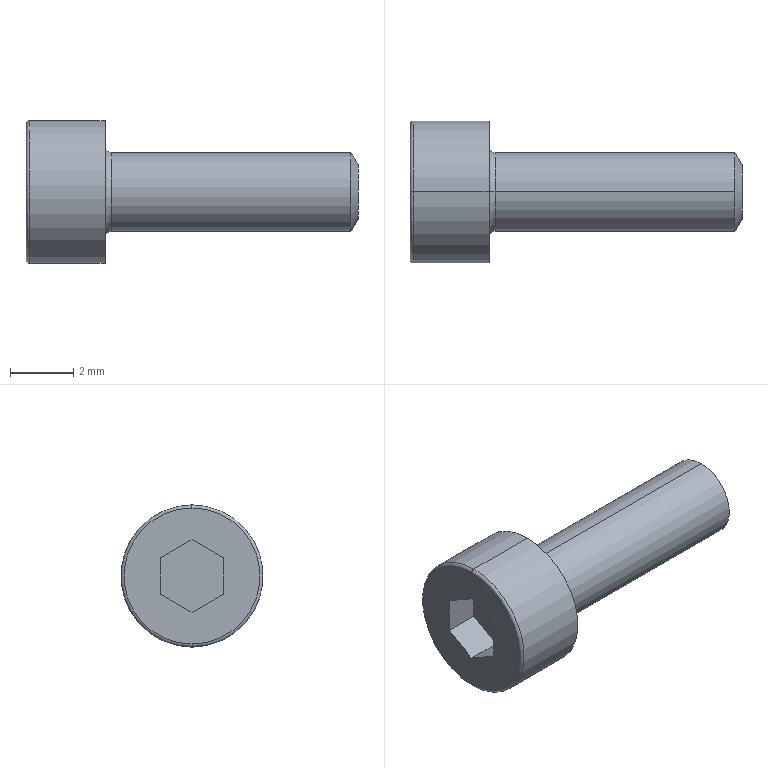Part | SolidWorks | features BlendCut 1, Cut 1, Fillet 1, LPattern 1, RevCut 1, Revolution 1 | 1 solid | 20 faces | box 10.5 x 4.5 x 4.5 mm | volume 74.982 mm3 | plane 10 | torus 4 | cylinder 4 | cone 2 | commonest cylinder face diameters 2.5 x2 4.5 x2
STEP:
#1=CARTESIAN_POINT('',(0.,0.,2.15));
#2=VERTEX_POINT('',#1);
#3=CARTESIAN_POINT('',(0.,0.,-2.15));
#4=VERTEX_POINT('',#3);
#5=CARTESIAN_POINT('',(0.,0.,0.));
#6=DIRECTION('',(-1.,0.,0.));
#7=DIRECTION('',(0.,0.,-1.));
#8=AXIS2_PLACEMENT_3D('',#5,#6,#7);
#9=CIRCLE('',#8,2.15);
#10=EDGE_CURVE('',#2,#4,#9,.T.);
#11=ORIENTED_EDGE('',*,*,#10,.F.);
#12=CARTESIAN_POINT('',(0.1,0.,2.25));
#13=VERTEX_POINT('',#12);
#14=CARTESIAN_POINT('',(0.1,0.,2.15));
#15=DIRECTION('',(0.,1.,0.));
#16=DIRECTION('',(0.,0.,1.));
#17=AXIS2_PLACEMENT_3D('',#14,#15,#16);
#18=CIRCLE('',#17,0.1);
#19=EDGE_CURVE('',#2,#13,#18,.T.);
#20=ORIENTED_EDGE('',*,*,#19,.T.);
#21=CARTESIAN_POINT('',(0.1,0.,-2.25));
#22=VERTEX_POINT('',#21);
#23=CARTESIAN_POINT('',(0.1,0.,0.));
#24=DIRECTION('',(1.,0.,0.));
#25=DIRECTION('',(0.,0.,-1.));
#26=AXIS2_PLACEMENT_3D('',#23,#24,#25);
#27=CIRCLE('',#26,2.25);
#28=EDGE_CURVE('',#22,#13,#27,.T.);
#29=ORIENTED_EDGE('',*,*,#28,.F.);
#30=CARTESIAN_POINT('',(0.1,0.,-2.15));
#31=DIRECTION('',(0.,-1.,0.));
#32=DIRECTION('',(0.,0.,-1.));
#33=AXIS2_PLACEMENT_3D('',#30,#31,#32);
#34=CIRCLE('',#33,0.1);
#35=EDGE_CURVE('',#4,#22,#34,.T.);
#36=ORIENTED_EDGE('',*,*,#35,.F.);
#37=EDGE_LOOP('',(#11,#20,#29,#36));
#38=FACE_OUTER_BOUND('',#37,.T.);
#39=CARTESIAN_POINT('',(0.1,0.,0.));
#40=DIRECTION('',(1.,0.,0.));
#41=DIRECTION('',(0.,0.,-1.));
#42=AXIS2_PLACEMENT_3D('',#39,#40,#41);
#43=TOROIDAL_SURFACE('',#42,2.15,0.1);
#44=ADVANCED_FACE('',(#38),#43,.T.);
#45=CARTESIAN_POINT('',(10.5,0.,0.8603));
#46=VERTEX_POINT('',#45);
#47=CARTESIAN_POINT('',(10.5,0.,-0.8603));
#48=VERTEX_POINT('',#47);
#49=CARTESIAN_POINT('',(10.5,0.,0.));
#50=DIRECTION('',(-1.,0.,0.));
#51=DIRECTION('',(0.,0.,1.));
#52=AXIS2_PLACEMENT_3D('',#49,#50,#51);
#53=CIRCLE('',#52,0.8603);
#54=EDGE_CURVE('',#46,#48,#53,.T.);
#55=ORIENTED_EDGE('',*,*,#54,.T.);
#56=CARTESIAN_POINT('',(10.275,0.,-1.25));
#57=VERTEX_POINT('',#56);
#58=CARTESIAN_POINT('',(10.275,0.,-1.25));
#59=DIRECTION('',(-0.5,0.,-0.866));
#60=VECTOR('',#59,1000.);
#61=LINE('',#58,#60);
#62=EDGE_CURVE('',#48,#57,#61,.T.);
#63=ORIENTED_EDGE('',*,*,#62,.T.);
#64=CARTESIAN_POINT('',(10.275,0.,1.25));
#65=VERTEX_POINT('',#64);
#66=CARTESIAN_POINT('',(10.275,0.,0.));
#67=DIRECTION('',(-1.,0.,0.));
#68=DIRECTION('',(0.,0.,1.));
#69=AXIS2_PLACEMENT_3D('',#66,#67,#68);
#70=CIRCLE('',#69,1.25);
#71=EDGE_CURVE('',#65,#57,#70,.T.);
#72=ORIENTED_EDGE('',*,*,#71,.F.);
#73=CARTESIAN_POINT('',(10.275,0.,1.25));
#74=DIRECTION('',(-0.5,0.,0.866));
#75=VECTOR('',#74,1000.);
#76=LINE('',#73,#75);
#77=EDGE_CURVE('',#46,#65,#76,.T.);
#78=ORIENTED_EDGE('',*,*,#77,.F.);
#79=EDGE_LOOP('',(#55,#63,#72,#78));
#80=FACE_OUTER_BOUND('',#79,.T.);
#81=CARTESIAN_POINT('',(10.275,0.,0.));
#82=DIRECTION('',(-1.,0.,0.));
#83=DIRECTION('',(0.,0.,1.));
#84=AXIS2_PLACEMENT_3D('',#81,#82,#83);
#85=CONICAL_SURFACE('',#84,1.25,1.047);
#86=ADVANCED_FACE('',(#80),#85,.T.);
#87=CARTESIAN_POINT('',(2.5,0.,-1.45));
#88=VERTEX_POINT('',#87);
#89=CARTESIAN_POINT('',(2.5,0.,1.45));
#90=VERTEX_POINT('',#89);
#91=CARTESIAN_POINT('',(2.5,0.,0.));
#92=DIRECTION('',(-1.,0.,0.));
#93=DIRECTION('',(0.,0.,1.));
#94=AXIS2_PLACEMENT_3D('',#91,#92,#93);
#95=CIRCLE('',#94,1.45);
#96=EDGE_CURVE('',#88,#90,#95,.T.);
#97=ORIENTED_EDGE('',*,*,#96,.F.);
#98=CARTESIAN_POINT('',(2.7,0.,-1.25));
#99=VERTEX_POINT('',#98);
#100=CARTESIAN_POINT('',(2.7,0.,-1.45));
#101=DIRECTION('',(0.,1.,0.));
#102=DIRECTION('',(0.,0.,1.));
#103=AXIS2_PLACEMENT_3D('',#100,#101,#102);
#104=CIRCLE('',#103,0.2);
#105=EDGE_CURVE('',#88,#99,#104,.T.);
#106=ORIENTED_EDGE('',*,*,#105,.T.);
#107=CARTESIAN_POINT('',(2.7,0.,1.25));
#108=VERTEX_POINT('',#107);
#109=CARTESIAN_POINT('',(2.7,0.,0.));
#110=DIRECTION('',(-1.,0.,0.));
#111=DIRECTION('',(0.,0.,1.));
#112=AXIS2_PLACEMENT_3D('',#109,#110,#111);
#113=CIRCLE('',#112,1.25);
#114=EDGE_CURVE('',#99,#108,#113,.T.);
#115=ORIENTED_EDGE('',*,*,#114,.T.);
#116=CARTESIAN_POINT('',(2.7,0.,1.45));
#117=DIRECTION('',(0.,-1.,0.));
#118=DIRECTION('',(0.,0.,-1.));
#119=AXIS2_PLACEMENT_3D('',#116,#117,#118);
#120=CIRCLE('',#119,0.2);
#121=EDGE_CURVE('',#90,#108,#120,.T.);
#122=ORIENTED_EDGE('',*,*,#121,.F.);
#123=EDGE_LOOP('',(#97,#106,#115,#122));
#124=FACE_OUTER_BOUND('',#123,.T.);
#125=CARTESIAN_POINT('',(2.7,0.,0.));
#126=DIRECTION('',(-1.,0.,0.));
#127=DIRECTION('',(0.,0.,1.));
#128=AXIS2_PLACEMENT_3D('',#125,#126,#127);
#129=TOROIDAL_SURFACE('',#128,1.45,0.2);
#130=ADVANCED_FACE('',(#124),#129,.F.);
#131=CARTESIAN_POINT('',(2.5,0.,2.25));
#132=VERTEX_POINT('',#131);
#133=CARTESIAN_POINT('',(2.5,0.,-2.25));
#134=VERTEX_POINT('',#133);
#135=CARTESIAN_POINT('',(2.5,0.,0.));
#136=DIRECTION('',(-1.,0.,0.));
#137=DIRECTION('',(0.,0.,1.));
#138=AXIS2_PLACEMENT_3D('',#135,#136,#137);
#139=CIRCLE('',#138,2.25);
#140=EDGE_CURVE('',#132,#134,#139,.T.);
#141=ORIENTED_EDGE('',*,*,#140,.T.);
#142=CARTESIAN_POINT('',(0.,0.,-2.25));
#143=DIRECTION('',(-1.,0.,0.));
#144=VECTOR('',#143,1000.);
#145=LINE('',#142,#144);
#146=EDGE_CURVE('',#134,#22,#145,.T.);
#147=ORIENTED_EDGE('',*,*,#146,.T.);
#148=ORIENTED_EDGE('',*,*,#28,.T.);
#149=CARTESIAN_POINT('',(0.,0.,2.25));
#150=DIRECTION('',(-1.,0.,0.));
#151=VECTOR('',#150,1000.);
#152=LINE('',#149,#151);
#153=EDGE_CURVE('',#132,#13,#152,.T.);
#154=ORIENTED_EDGE('',*,*,#153,.F.);
#155=EDGE_LOOP('',(#141,#147,#148,#154));
#156=FACE_OUTER_BOUND('',#155,.T.);
#157=CARTESIAN_POINT('',(0.,0.,0.));
#158=DIRECTION('',(-1.,0.,0.));
#159=DIRECTION('',(0.,0.,1.));
#160=AXIS2_PLACEMENT_3D('',#157,#158,#159);
#161=CYLINDRICAL_SURFACE('',#160,2.25);
#162=ADVANCED_FACE('',(#156),#161,.T.);
#163=ORIENTED_EDGE('',*,*,#71,.T.);
#164=CARTESIAN_POINT('',(0.,0.,-1.25));
#165=DIRECTION('',(-1.,0.,0.));
#166=VECTOR('',#165,1000.);
#167=LINE('',#164,#166);
#168=EDGE_CURVE('',#57,#99,#167,.T.);
#169=ORIENTED_EDGE('',*,*,#168,.T.);
#170=CARTESIAN_POINT('',(2.7,0.,0.));
#171=DIRECTION('',(-1.,0.,0.));
#172=DIRECTION('',(0.,0.,1.));
#173=AXIS2_PLACEMENT_3D('',#170,#171,#172);
#174=CIRCLE('',#173,1.25);
#175=EDGE_CURVE('',#108,#99,#174,.T.);
#176=ORIENTED_EDGE('',*,*,#175,.F.);
#177=CARTESIAN_POINT('',(0.,0.,1.25));
#178=DIRECTION('',(-1.,0.,0.));
#179=VECTOR('',#178,1000.);
#180=LINE('',#177,#179);
#181=EDGE_CURVE('',#65,#108,#180,.T.);
#182=ORIENTED_EDGE('',*,*,#181,.F.);
#183=EDGE_LOOP('',(#163,#169,#176,#182));
#184=FACE_OUTER_BOUND('',#183,.T.);
#185=CARTESIAN_POINT('',(0.,0.,0.));
#186=DIRECTION('',(-1.,0.,0.));
#187=DIRECTION('',(0.,0.,1.));
#188=AXIS2_PLACEMENT_3D('',#185,#186,#187);
#189=CYLINDRICAL_SURFACE('',#188,1.25);
#190=ADVANCED_FACE('',(#184),#189,.T.);
#191=ORIENTED_EDGE('',*,*,#168,.F.);
#192=CARTESIAN_POINT('',(10.275,0.,0.));
#193=DIRECTION('',(-1.,0.,0.));
#194=DIRECTION('',(0.,0.,1.));
#195=AXIS2_PLACEMENT_3D('',#192,#193,#194);
#196=CIRCLE('',#195,1.25);
#197=EDGE_CURVE('',#57,#65,#196,.T.);
#198=ORIENTED_EDGE('',*,*,#197,.T.);
#199=ORIENTED_EDGE('',*,*,#181,.T.);
#200=ORIENTED_EDGE('',*,*,#114,.F.);
#201=EDGE_LOOP('',(#191,#198,#199,#200));
#202=FACE_OUTER_BOUND('',#201,.T.);
#203=CARTESIAN_POINT('',(0.,0.,0.));
#204=DIRECTION('',(-1.,0.,0.));
#205=DIRECTION('',(0.,0.,1.));
#206=AXIS2_PLACEMENT_3D('',#203,#204,#205);
#207=CYLINDRICAL_SURFACE('',#206,1.25);
#208=ADVANCED_FACE('',(#202),#207,.T.);
#209=CARTESIAN_POINT('',(0.,0.,0.));
#210=DIRECTION('',(-1.,0.,0.));
#211=DIRECTION('',(0.,0.,-1.));
#212=AXIS2_PLACEMENT_3D('',#209,#210,#211);
#213=CIRCLE('',#212,2.15);
#214=EDGE_CURVE('',#4,#2,#213,.T.);
#215=ORIENTED_EDGE('',*,*,#214,.T.);
#216=ORIENTED_EDGE('',*,*,#10,.T.);
#217=EDGE_LOOP('',(#215,#216));
#218=FACE_OUTER_BOUND('',#217,.T.);
#219=CARTESIAN_POINT('',(0.,0.,1.15));
#220=VERTEX_POINT('',#219);
#221=CARTESIAN_POINT('',(0.,0.9959,0.575));
#222=VERTEX_POINT('',#221);
#223=CARTESIAN_POINT('',(0.,0.,1.15));
#224=DIRECTION('',(0.,0.866,-0.5));
#225=VECTOR('',#224,1000.);
#226=LINE('',#223,#225);
#227=EDGE_CURVE('',#220,#222,#226,.T.);
#228=ORIENTED_EDGE('',*,*,#227,.F.);
#229=CARTESIAN_POINT('',(0.,-0.9959,0.575));
#230=VERTEX_POINT('',#229);
#231=CARTESIAN_POINT('',(0.,-0.9959,0.575));
#232=DIRECTION('',(0.,0.866,0.5));
#233=VECTOR('',#232,1000.);
#234=LINE('',#231,#233);
#235=EDGE_CURVE('',#230,#220,#234,.T.);
#236=ORIENTED_EDGE('',*,*,#235,.F.);
#237=CARTESIAN_POINT('',(0.,-0.9959,-0.575));
#238=VERTEX_POINT('',#237);
#239=CARTESIAN_POINT('',(0.,-0.9959,-0.575));
#240=DIRECTION('',(0.,0.,1.));
#241=VECTOR('',#240,1000.);
#242=LINE('',#239,#241);
#243=EDGE_CURVE('',#238,#230,#242,.T.);
#244=ORIENTED_EDGE('',*,*,#243,.F.);
#245=CARTESIAN_POINT('',(0.,0.,-1.15));
#246=VERTEX_POINT('',#245);
#247=CARTESIAN_POINT('',(0.,0.,-1.15));
#248=DIRECTION('',(0.,-0.866,0.5));
#249=VECTOR('',#248,1000.);
#250=LINE('',#247,#249);
#251=EDGE_CURVE('',#246,#238,#250,.T.);
#252=ORIENTED_EDGE('',*,*,#251,.F.);
#253=CARTESIAN_POINT('',(0.,0.9959,-0.575));
#254=VERTEX_POINT('',#253);
#255=CARTESIAN_POINT('',(0.,0.9959,-0.575));
#256=DIRECTION('',(0.,-0.866,-0.5));
#257=VECTOR('',#256,1000.);
#258=LINE('',#255,#257);
#259=EDGE_CURVE('',#254,#246,#258,.T.);
#260=ORIENTED_EDGE('',*,*,#259,.F.);
#261=CARTESIAN_POINT('',(0.,0.9959,0.575));
#262=DIRECTION('',(0.,0.,-1.));
#263=VECTOR('',#262,1000.);
#264=LINE('',#261,#263);
#265=EDGE_CURVE('',#222,#254,#264,.T.);
#266=ORIENTED_EDGE('',*,*,#265,.F.);
#267=EDGE_LOOP('',(#228,#236,#244,#252,#260,#266));
#268=FACE_BOUND('',#267,.T.);
#269=CARTESIAN_POINT('',(0.,0.,0.));
#270=DIRECTION('',(1.,0.,0.));
#271=DIRECTION('',(0.,0.,-1.));
#272=AXIS2_PLACEMENT_3D('',#269,#270,#271);
#273=PLANE('',#272);
#274=ADVANCED_FACE('',(#218,#268),#273,.F.);
#275=ORIENTED_EDGE('',*,*,#146,.F.);
#276=CARTESIAN_POINT('',(2.5,0.,0.));
#277=DIRECTION('',(-1.,0.,0.));
#278=DIRECTION('',(0.,0.,1.));
#279=AXIS2_PLACEMENT_3D('',#276,#277,#278);
#280=CIRCLE('',#279,2.25);
#281=EDGE_CURVE('',#134,#132,#280,.T.);
#282=ORIENTED_EDGE('',*,*,#281,.T.);
#283=ORIENTED_EDGE('',*,*,#153,.T.);
#284=CARTESIAN_POINT('',(0.1,0.,0.));
#285=DIRECTION('',(1.,0.,0.));
#286=DIRECTION('',(0.,0.,-1.));
#287=AXIS2_PLACEMENT_3D('',#284,#285,#286);
#288=CIRCLE('',#287,2.25);
#289=EDGE_CURVE('',#13,#22,#288,.T.);
#290=ORIENTED_EDGE('',*,*,#289,.T.);
#291=EDGE_LOOP('',(#275,#282,#283,#290));
#292=FACE_OUTER_BOUND('',#291,.T.);
#293=CARTESIAN_POINT('',(0.,0.,0.));
#294=DIRECTION('',(-1.,0.,0.));
#295=DIRECTION('',(0.,0.,1.));
#296=AXIS2_PLACEMENT_3D('',#293,#294,#295);
#297=CYLINDRICAL_SURFACE('',#296,2.25);
#298=ADVANCED_FACE('',(#292),#297,.T.);
#299=ORIENTED_EDGE('',*,*,#140,.F.);
#300=ORIENTED_EDGE('',*,*,#281,.F.);
#301=EDGE_LOOP('',(#299,#300));
#302=FACE_OUTER_BOUND('',#301,.T.);
#303=CARTESIAN_POINT('',(2.5,0.,0.));
#304=DIRECTION('',(-1.,0.,0.));
#305=DIRECTION('',(0.,0.,1.));
#306=AXIS2_PLACEMENT_3D('',#303,#304,#305);
#307=CIRCLE('',#306,1.45);
#308=EDGE_CURVE('',#90,#88,#307,.T.);
#309=ORIENTED_EDGE('',*,*,#308,.T.);
#310=ORIENTED_EDGE('',*,*,#96,.T.);
#311=EDGE_LOOP('',(#309,#310));
#312=FACE_BOUND('',#311,.T.);
#313=CARTESIAN_POINT('',(2.5,2.25,0.));
#314=DIRECTION('',(-1.,0.,0.));
#315=DIRECTION('',(0.,0.,1.));
#316=AXIS2_PLACEMENT_3D('',#313,#314,#315);
#317=PLANE('',#316);
#318=ADVANCED_FACE('',(#302,#312),#317,.F.);
#319=ORIENTED_EDGE('',*,*,#105,.F.);
#320=ORIENTED_EDGE('',*,*,#308,.F.);
#321=ORIENTED_EDGE('',*,*,#121,.T.);
#322=ORIENTED_EDGE('',*,*,#175,.T.);
#323=EDGE_LOOP('',(#319,#320,#321,#322));
#324=FACE_OUTER_BOUND('',#323,.T.);
#325=CARTESIAN_POINT('',(2.7,0.,0.));
#326=DIRECTION('',(-1.,0.,0.));
#327=DIRECTION('',(0.,0.,1.));
#328=AXIS2_PLACEMENT_3D('',#325,#326,#327);
#329=TOROIDAL_SURFACE('',#328,1.45,0.2);
#330=ADVANCED_FACE('',(#324),#329,.F.);
#331=ORIENTED_EDGE('',*,*,#235,.T.);
#332=CARTESIAN_POINT('',(1.1,0.,1.15));
#333=VERTEX_POINT('',#332);
#334=CARTESIAN_POINT('',(1.1,0.,1.15));
#335=DIRECTION('',(-1.,0.,0.));
#336=VECTOR('',#335,1000.);
#337=LINE('',#334,#336);
#338=EDGE_CURVE('',#333,#220,#337,.T.);
#339=ORIENTED_EDGE('',*,*,#338,.F.);
#340=CARTESIAN_POINT('',(1.1,-0.9959,0.575));
#341=VERTEX_POINT('',#340);
#342=CARTESIAN_POINT('',(1.1,-0.9959,0.575));
#343=DIRECTION('',(0.,0.866,0.5));
#344=VECTOR('',#343,1000.);
#345=LINE('',#342,#344);
#346=EDGE_CURVE('',#341,#333,#345,.T.);
#347=ORIENTED_EDGE('',*,*,#346,.F.);
#348=CARTESIAN_POINT('',(1.1,-0.9959,0.575));
#349=DIRECTION('',(-1.,0.,0.));
#350=VECTOR('',#349,1000.);
#351=LINE('',#348,#350);
#352=EDGE_CURVE('',#341,#230,#351,.T.);
#353=ORIENTED_EDGE('',*,*,#352,.T.);
#354=EDGE_LOOP('',(#331,#339,#347,#353));
#355=FACE_OUTER_BOUND('',#354,.T.);
#356=CARTESIAN_POINT('',(1.1,-0.9959,0.575));
#357=DIRECTION('',(0.,-0.5,0.866));
#358=DIRECTION('',(0.,-0.866,-0.5));
#359=AXIS2_PLACEMENT_3D('',#356,#357,#358);
#360=PLANE('',#359);
#361=ADVANCED_FACE('',(#355),#360,.F.);
#362=ORIENTED_EDGE('',*,*,#243,.T.);
#363=ORIENTED_EDGE('',*,*,#352,.F.);
#364=CARTESIAN_POINT('',(1.1,-0.9959,-0.575));
#365=VERTEX_POINT('',#364);
#366=CARTESIAN_POINT('',(1.1,-0.9959,-0.575));
#367=DIRECTION('',(0.,0.,1.));
#368=VECTOR('',#367,1000.);
#369=LINE('',#366,#368);
#370=EDGE_CURVE('',#365,#341,#369,.T.);
#371=ORIENTED_EDGE('',*,*,#370,.F.);
#372=CARTESIAN_POINT('',(1.1,-0.9959,-0.575));
#373=DIRECTION('',(-1.,0.,0.));
#374=VECTOR('',#373,1000.);
#375=LINE('',#372,#374);
#376=EDGE_CURVE('',#365,#238,#375,.T.);
#377=ORIENTED_EDGE('',*,*,#376,.T.);
#378=EDGE_LOOP('',(#362,#363,#371,#377));
#379=FACE_OUTER_BOUND('',#378,.T.);
#380=CARTESIAN_POINT('',(1.1,-0.9959,-0.575));
#381=DIRECTION('',(0.,-1.,0.));
#382=DIRECTION('',(0.,0.,-1.));
#383=AXIS2_PLACEMENT_3D('',#380,#381,#382);
#384=PLANE('',#383);
#385=ADVANCED_FACE('',(#379),#384,.F.);
#386=ORIENTED_EDGE('',*,*,#251,.T.);
#387=ORIENTED_EDGE('',*,*,#376,.F.);
#388=CARTESIAN_POINT('',(1.1,0.,-1.15));
#389=VERTEX_POINT('',#388);
#390=CARTESIAN_POINT('',(1.1,0.,-1.15));
#391=DIRECTION('',(0.,-0.866,0.5));
#392=VECTOR('',#391,1000.);
#393=LINE('',#390,#392);
#394=EDGE_CURVE('',#389,#365,#393,.T.);
#395=ORIENTED_EDGE('',*,*,#394,.F.);
#396=CARTESIAN_POINT('',(1.1,0.,-1.15));
#397=DIRECTION('',(-1.,0.,0.));
#398=VECTOR('',#397,1000.);
#399=LINE('',#396,#398);
#400=EDGE_CURVE('',#389,#246,#399,.T.);
#401=ORIENTED_EDGE('',*,*,#400,.T.);
#402=EDGE_LOOP('',(#386,#387,#395,#401));
#403=FACE_OUTER_BOUND('',#402,.T.);
#404=CARTESIAN_POINT('',(1.1,0.,-1.15));
#405=DIRECTION('',(0.,-0.5,-0.866));
#406=DIRECTION('',(0.,0.866,-0.5));
#407=AXIS2_PLACEMENT_3D('',#404,#405,#406);
#408=PLANE('',#407);
#409=ADVANCED_FACE('',(#403),#408,.F.);
#410=ORIENTED_EDGE('',*,*,#259,.T.);
#411=ORIENTED_EDGE('',*,*,#400,.F.);
#412=CARTESIAN_POINT('',(1.1,0.9959,-0.575));
#413=VERTEX_POINT('',#412);
#414=CARTESIAN_POINT('',(1.1,0.9959,-0.575));
#415=DIRECTION('',(0.,-0.866,-0.5));
#416=VECTOR('',#415,1000.);
#417=LINE('',#414,#416);
#418=EDGE_CURVE('',#413,#389,#417,.T.);
#419=ORIENTED_EDGE('',*,*,#418,.F.);
#420=CARTESIAN_POINT('',(1.1,0.9959,-0.575));
#421=DIRECTION('',(-1.,0.,0.));
#422=VECTOR('',#421,1000.);
#423=LINE('',#420,#422);
#424=EDGE_CURVE('',#413,#254,#423,.T.);
#425=ORIENTED_EDGE('',*,*,#424,.T.);
#426=EDGE_LOOP('',(#410,#411,#419,#425));
#427=FACE_OUTER_BOUND('',#426,.T.);
#428=CARTESIAN_POINT('',(1.1,0.9959,-0.575));
#429=DIRECTION('',(0.,0.5,-0.866));
#430=DIRECTION('',(0.,0.866,0.5));
#431=AXIS2_PLACEMENT_3D('',#428,#429,#430);
#432=PLANE('',#431);
#433=ADVANCED_FACE('',(#427),#432,.F.);
#434=ORIENTED_EDGE('',*,*,#265,.T.);
#435=ORIENTED_EDGE('',*,*,#424,.F.);
#436=CARTESIAN_POINT('',(1.1,0.9959,0.575));
#437=VERTEX_POINT('',#436);
#438=CARTESIAN_POINT('',(1.1,0.9959,0.575));
#439=DIRECTION('',(0.,0.,-1.));
#440=VECTOR('',#439,1000.);
#441=LINE('',#438,#440);
#442=EDGE_CURVE('',#437,#413,#441,.T.);
#443=ORIENTED_EDGE('',*,*,#442,.F.);
#444=CARTESIAN_POINT('',(1.1,0.9959,0.575));
#445=DIRECTION('',(-1.,0.,0.));
#446=VECTOR('',#445,1000.);
#447=LINE('',#444,#446);
#448=EDGE_CURVE('',#437,#222,#447,.T.);
#449=ORIENTED_EDGE('',*,*,#448,.T.);
#450=EDGE_LOOP('',(#434,#435,#443,#449));
#451=FACE_OUTER_BOUND('',#450,.T.);
#452=CARTESIAN_POINT('',(1.1,0.9959,0.575));
#453=DIRECTION('',(0.,1.,0.));
#454=DIRECTION('',(0.,0.,1.));
#455=AXIS2_PLACEMENT_3D('',#452,#453,#454);
#456=PLANE('',#455);
#457=ADVANCED_FACE('',(#451),#456,.F.);
#458=ORIENTED_EDGE('',*,*,#227,.T.);
#459=ORIENTED_EDGE('',*,*,#448,.F.);
#460=CARTESIAN_POINT('',(1.1,0.,1.15));
#461=DIRECTION('',(0.,0.866,-0.5));
#462=VECTOR('',#461,1000.);
#463=LINE('',#460,#462);
#464=EDGE_CURVE('',#333,#437,#463,.T.);
#465=ORIENTED_EDGE('',*,*,#464,.F.);
#466=ORIENTED_EDGE('',*,*,#338,.T.);
#467=EDGE_LOOP('',(#458,#459,#465,#466));
#468=FACE_OUTER_BOUND('',#467,.T.);
#469=CARTESIAN_POINT('',(1.1,0.,1.15));
#470=DIRECTION('',(0.,0.5,0.866));
#471=DIRECTION('',(0.,-0.866,0.5));
#472=AXIS2_PLACEMENT_3D('',#469,#470,#471);
#473=PLANE('',#472);
#474=ADVANCED_FACE('',(#468),#473,.F.);
#475=ORIENTED_EDGE('',*,*,#346,.T.);
#476=ORIENTED_EDGE('',*,*,#464,.T.);
#477=ORIENTED_EDGE('',*,*,#442,.T.);
#478=ORIENTED_EDGE('',*,*,#418,.T.);
#479=ORIENTED_EDGE('',*,*,#394,.T.);
#480=ORIENTED_EDGE('',*,*,#370,.T.);
#481=EDGE_LOOP('',(#475,#476,#477,#478,#479,#480));
#482=FACE_OUTER_BOUND('',#481,.T.);
#483=CARTESIAN_POINT('',(1.1,-0.9959,0.575));
#484=DIRECTION('',(1.,0.,0.));
#485=DIRECTION('',(0.,0.,-1.));
#486=AXIS2_PLACEMENT_3D('',#483,#484,#485);
#487=PLANE('',#486);
#488=ADVANCED_FACE('',(#482),#487,.F.);
#489=ORIENTED_EDGE('',*,*,#62,.F.);
#490=CARTESIAN_POINT('',(10.5,0.,0.));
#491=DIRECTION('',(-1.,0.,0.));
#492=DIRECTION('',(0.,0.,1.));
#493=AXIS2_PLACEMENT_3D('',#490,#491,#492);
#494=CIRCLE('',#493,0.8603);
#495=EDGE_CURVE('',#48,#46,#494,.T.);
#496=ORIENTED_EDGE('',*,*,#495,.T.);
#497=ORIENTED_EDGE('',*,*,#77,.T.);
#498=ORIENTED_EDGE('',*,*,#197,.F.);
#499=EDGE_LOOP('',(#489,#496,#497,#498));
#500=FACE_OUTER_BOUND('',#499,.T.);
#501=CARTESIAN_POINT('',(10.275,0.,0.));
#502=DIRECTION('',(-1.,0.,0.));
#503=DIRECTION('',(0.,0.,1.));
#504=AXIS2_PLACEMENT_3D('',#501,#502,#503);
#505=CONICAL_SURFACE('',#504,1.25,1.047);
#506=ADVANCED_FACE('',(#500),#505,.T.);
#507=ORIENTED_EDGE('',*,*,#54,.F.);
#508=ORIENTED_EDGE('',*,*,#495,.F.);
#509=EDGE_LOOP('',(#507,#508));
#510=FACE_OUTER_BOUND('',#509,.T.);
#511=CARTESIAN_POINT('',(10.5,1.25,0.));
#512=DIRECTION('',(-1.,0.,0.));
#513=DIRECTION('',(0.,0.,1.));
#514=AXIS2_PLACEMENT_3D('',#511,#512,#513);
#515=PLANE('',#514);
#516=ADVANCED_FACE('',(#510),#515,.F.);
#517=ORIENTED_EDGE('',*,*,#19,.F.);
#518=ORIENTED_EDGE('',*,*,#214,.F.);
#519=ORIENTED_EDGE('',*,*,#35,.T.);
#520=ORIENTED_EDGE('',*,*,#289,.F.);
#521=EDGE_LOOP('',(#517,#518,#519,#520));
#522=FACE_OUTER_BOUND('',#521,.T.);
#523=CARTESIAN_POINT('',(0.1,0.,0.));
#524=DIRECTION('',(1.,0.,0.));
#525=DIRECTION('',(0.,0.,-1.));
#526=AXIS2_PLACEMENT_3D('',#523,#524,#525);
#527=TOROIDAL_SURFACE('',#526,2.15,0.1);
#528=ADVANCED_FACE('',(#522),#527,.T.);
#529=CLOSED_SHELL('',(#44,#86,#130,#162,#190,#208,#274,#298,#318,#330,#361,#385,#409,#433,#457,#474,#488,#506,#516,#528));
#530=MANIFOLD_SOLID_BREP('',#529);
#531=CARTESIAN_POINT('',(0.,0.,0.));
#532=DIRECTION('',(0.,0.,1.));
#533=DIRECTION('',(1.,0.,0.));
#534=AXIS2_PLACEMENT_3D('',#531,#532,#533);
#535=(LENGTH_UNIT()NAMED_UNIT(*)SI_UNIT(.MILLI.,.METRE.));
#536=UNCERTAINTY_MEASURE_WITH_UNIT(LENGTH_MEASURE(0.00001),#535,'','');
#537=(NAMED_UNIT(*)PLANE_ANGLE_UNIT()SI_UNIT($,.RADIAN.));
#538=(NAMED_UNIT(*)SI_UNIT($,.STERADIAN.)SOLID_ANGLE_UNIT());
#539=(GEOMETRIC_REPRESENTATION_CONTEXT(3)GLOBAL_UNCERTAINTY_ASSIGNED_CONTEXT((#536))GLOBAL_UNIT_ASSIGNED_CONTEXT((#535,#537,#538))REPRESENTATION_CONTEXT('',''));
#540=ADVANCED_BREP_SHAPE_REPRESENTATION('',(#530,#534),#539);